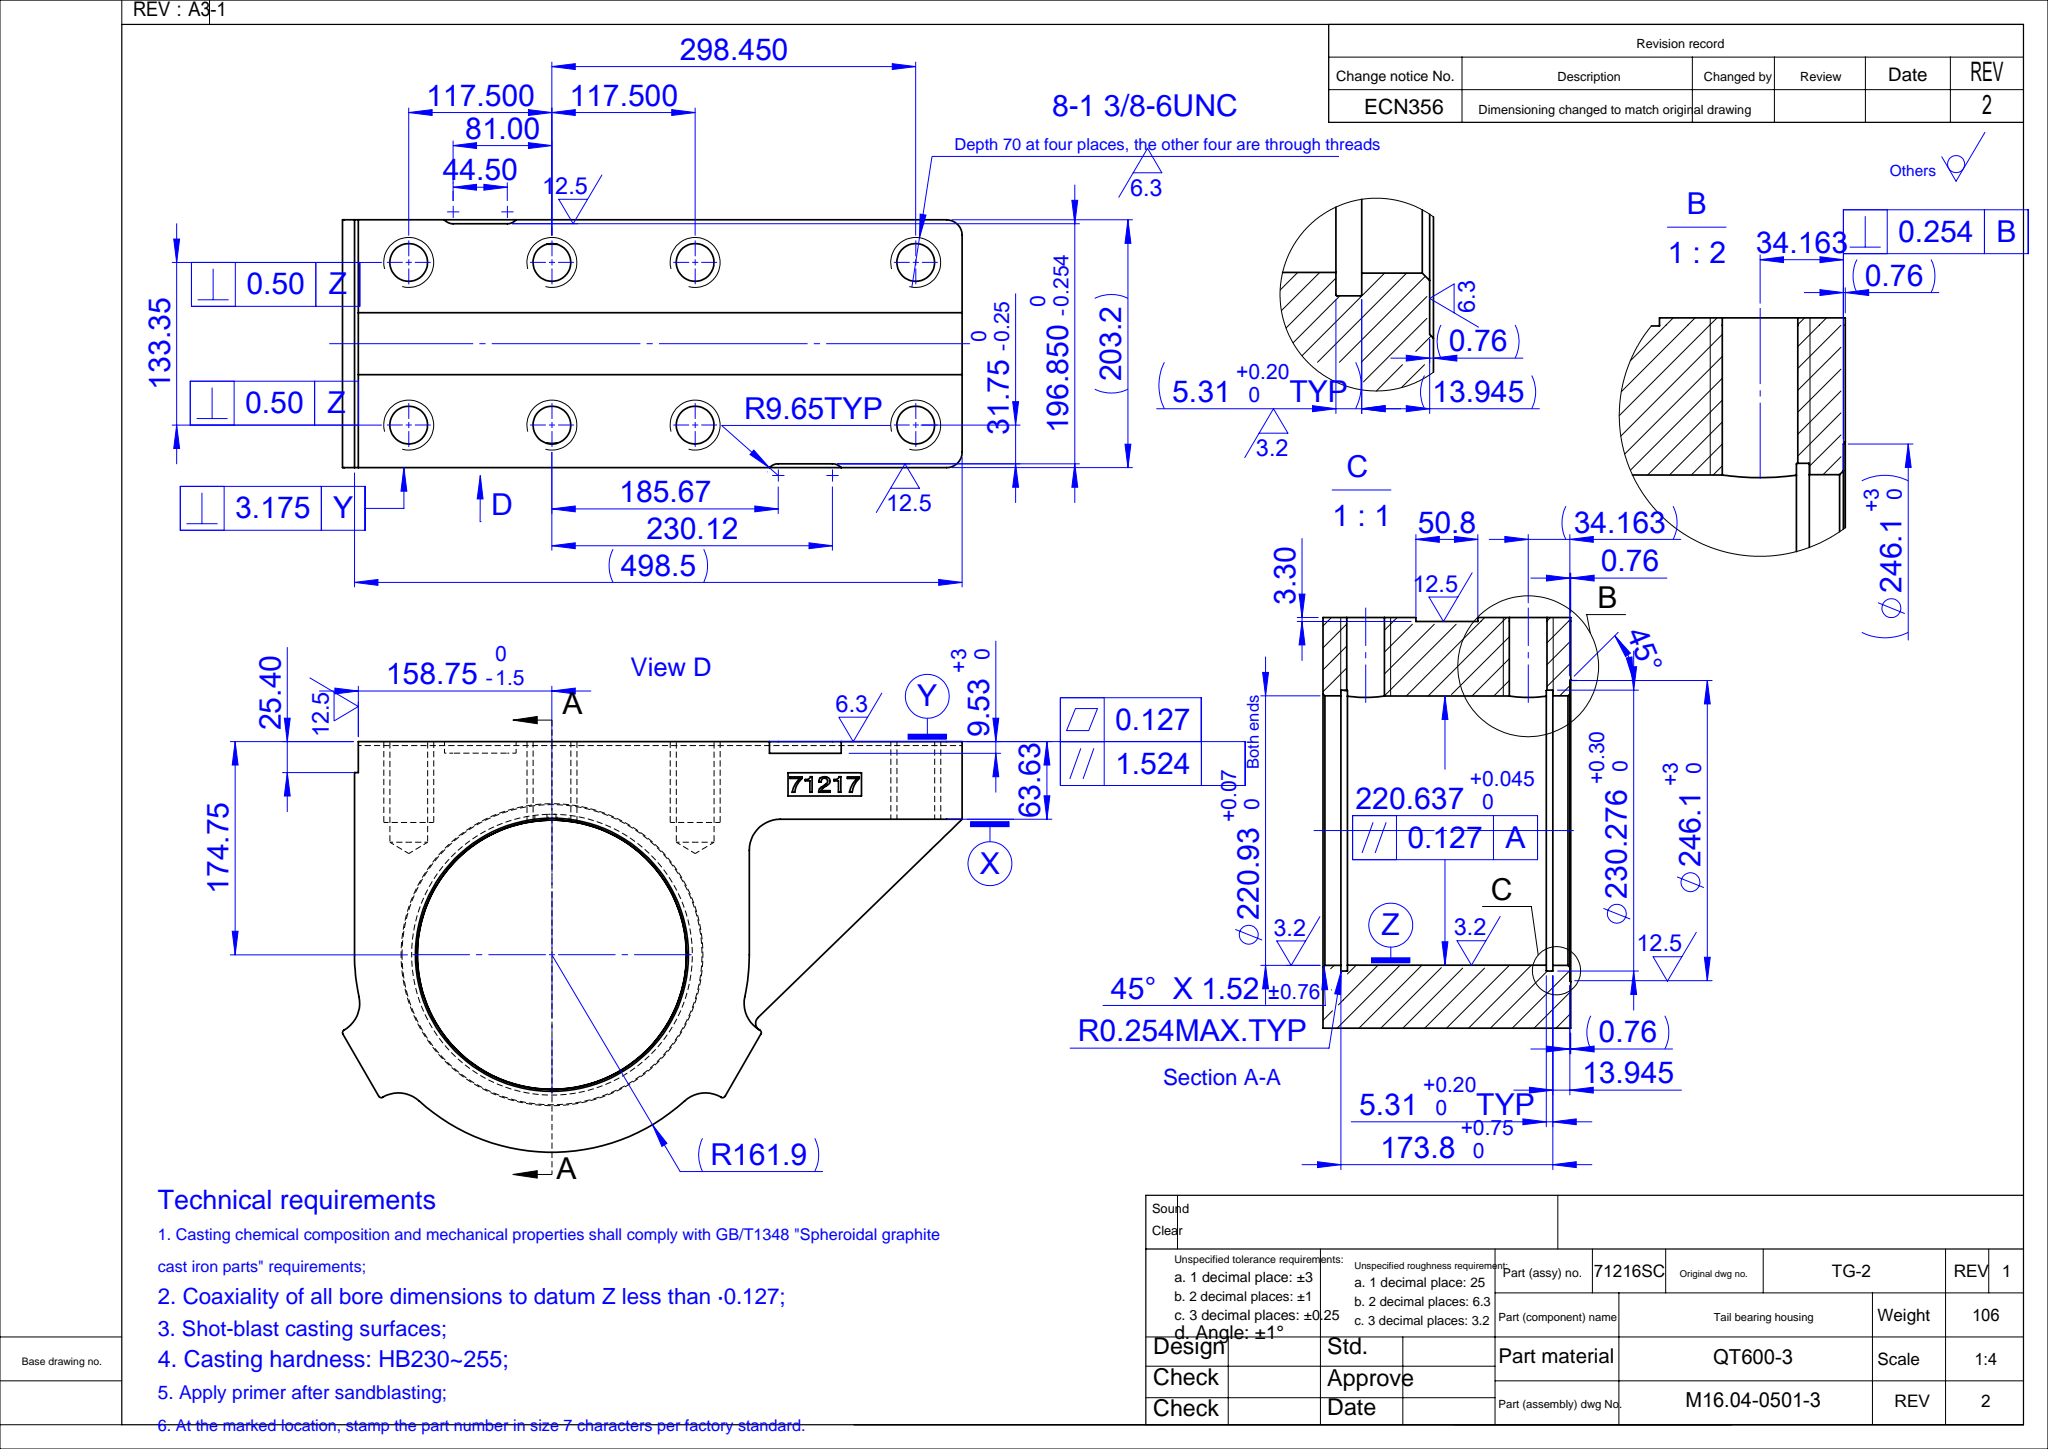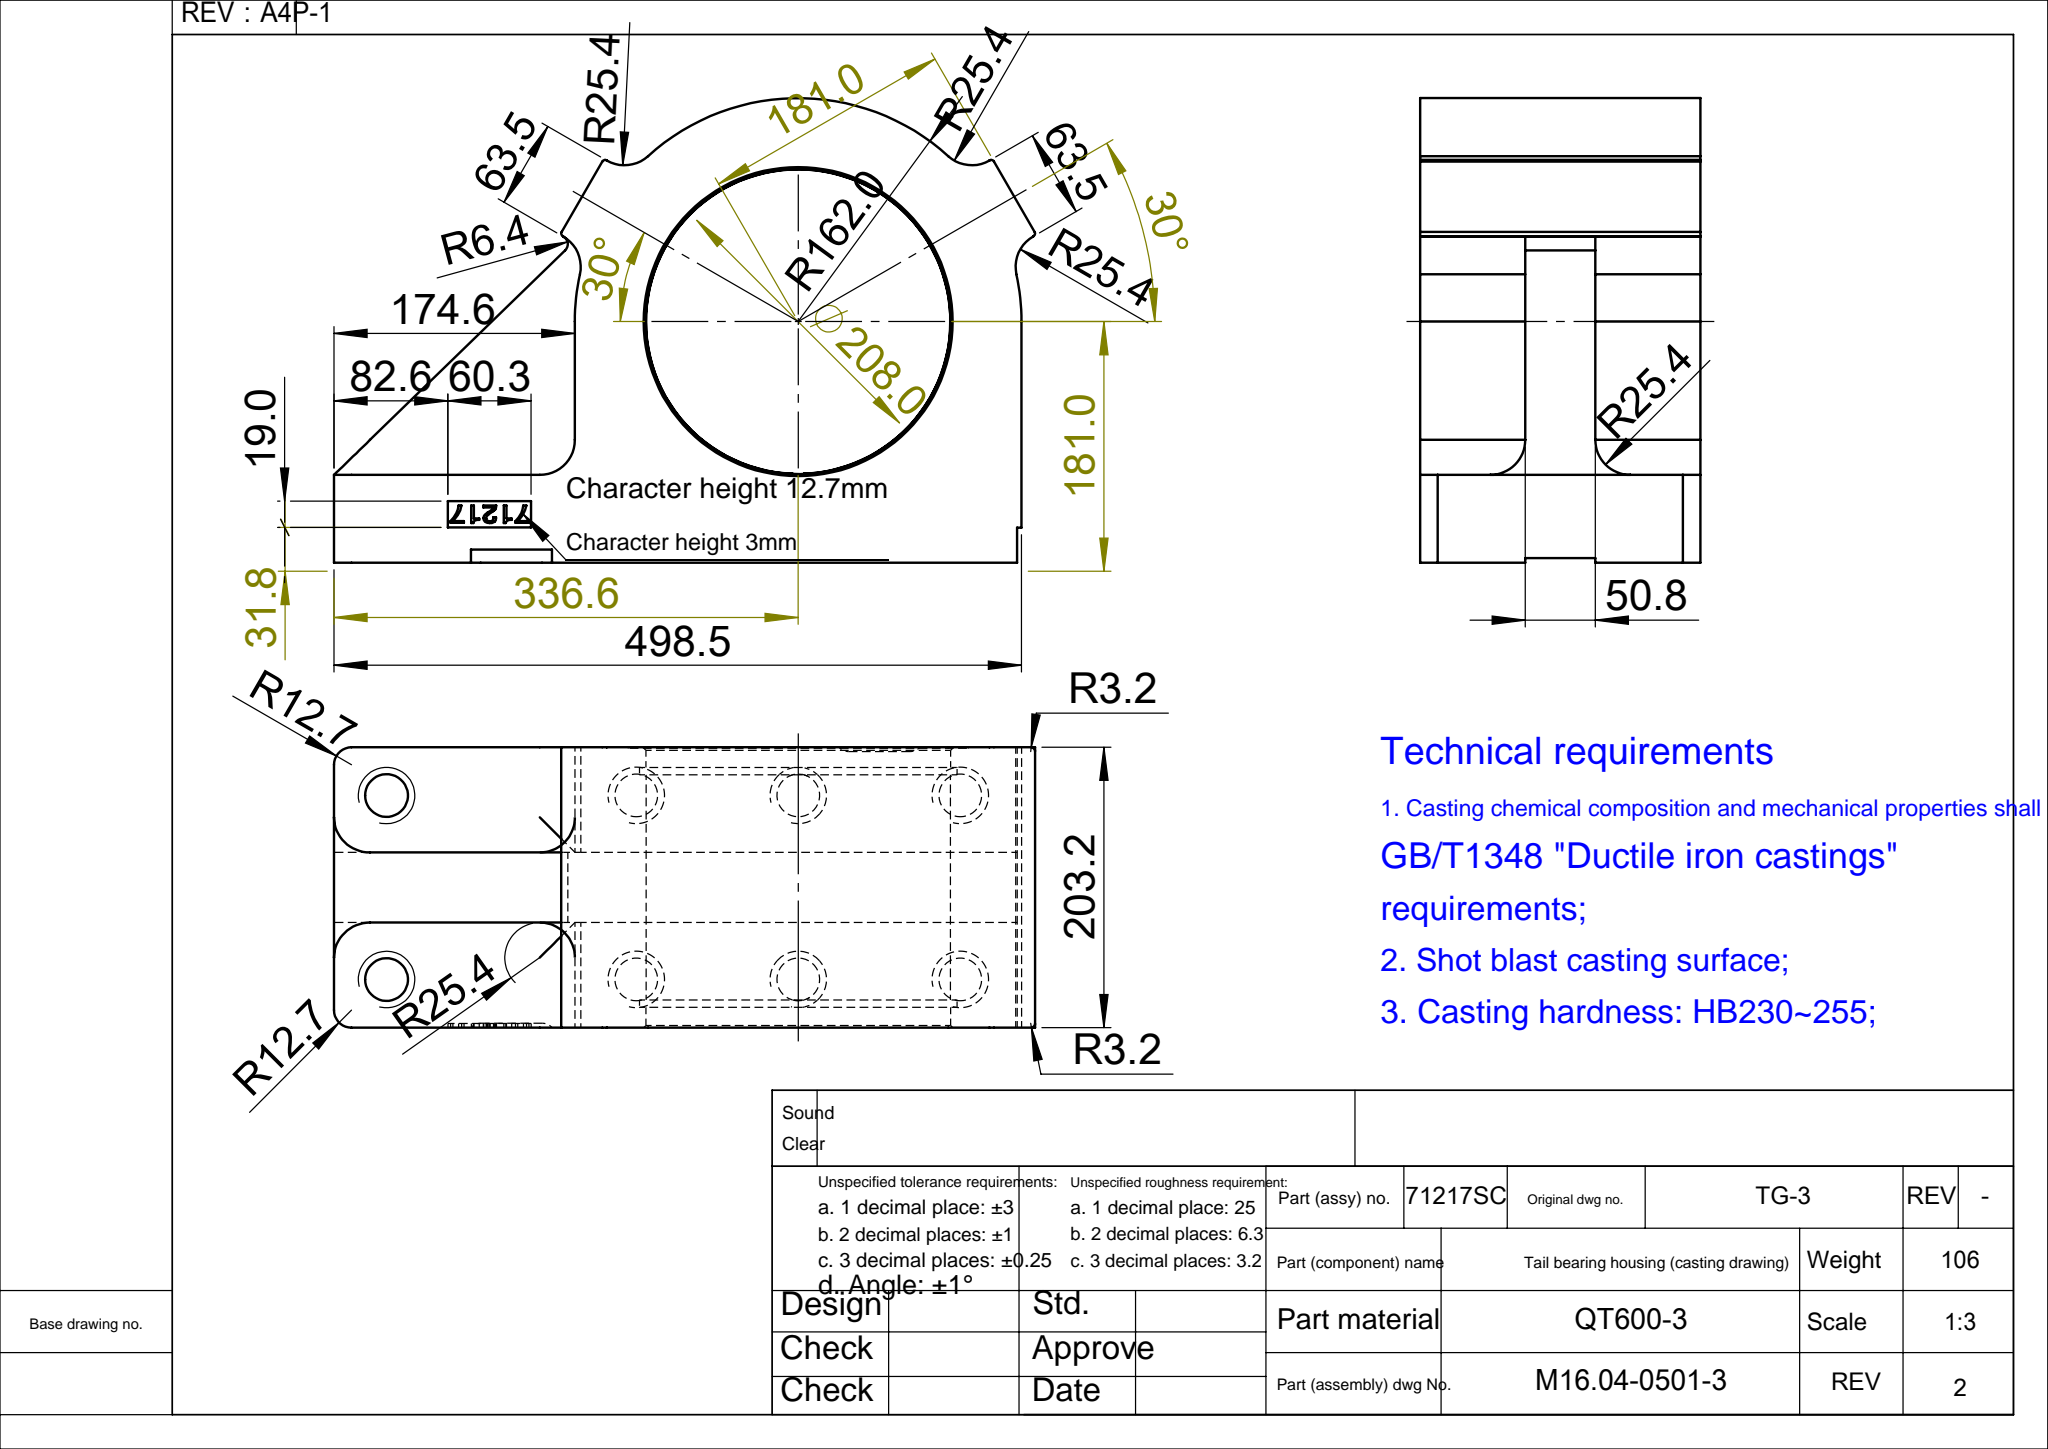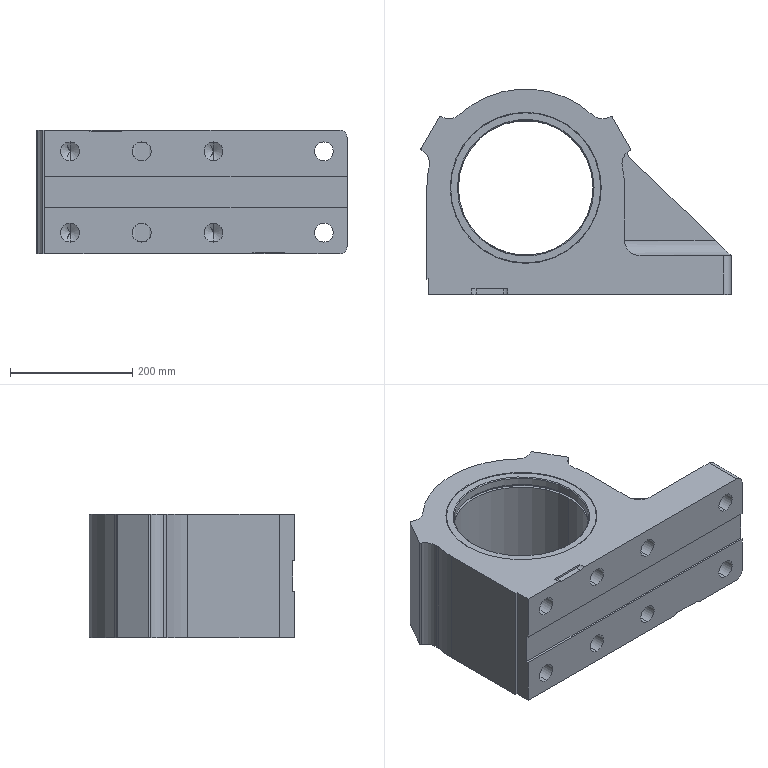Part | SolidWorks | features Fillet 5, Cut 4, Boss 3, Chamfer 2, 3DProfileFeature 1, HoleWzd 1, RevCut 1, Revolution 1, Rib 1, SketchPattern 1 | 1 solid | 163 faces | box 508.317 x 336.677 x 203.2 mm | volume 15145778 mm3 | plane 72 | cylinder 51 | spline 16 | cone 14 | torus 10 | commonest cylinder face diameters 30.958 x16 50.8 x9 4.572 x5 19.304 x4 220.929 x4 230.276 x4